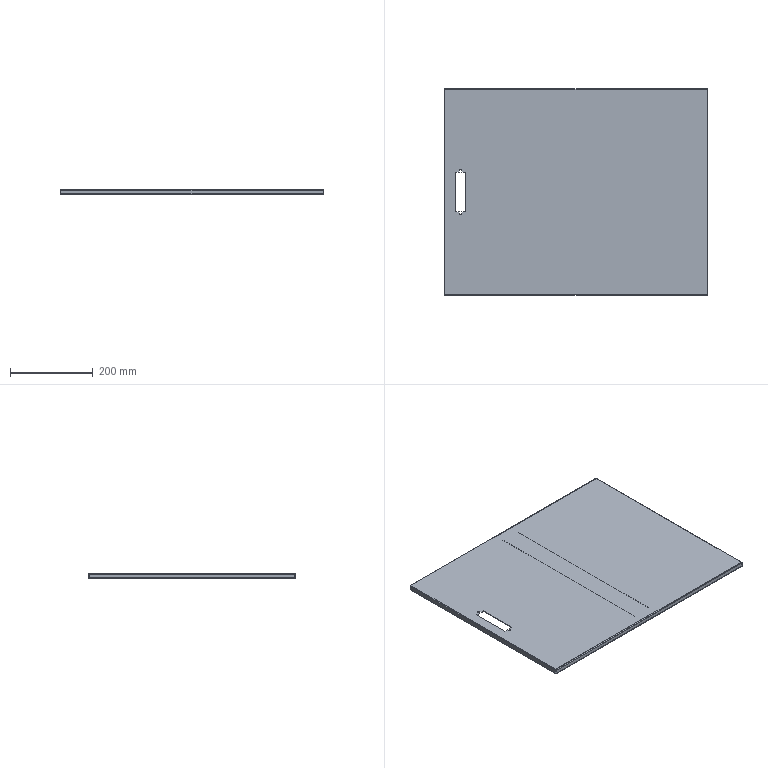Part | SolidWorks | features BaseBody 2 | 2 solids | 96 faces | box 638 x 500 x 13 mm | volume 600810 mm3 | plane 58 | cylinder 22 | spline 16 | commonest cylinder face diameters 1.473 x10 4.473 x10 6 x2